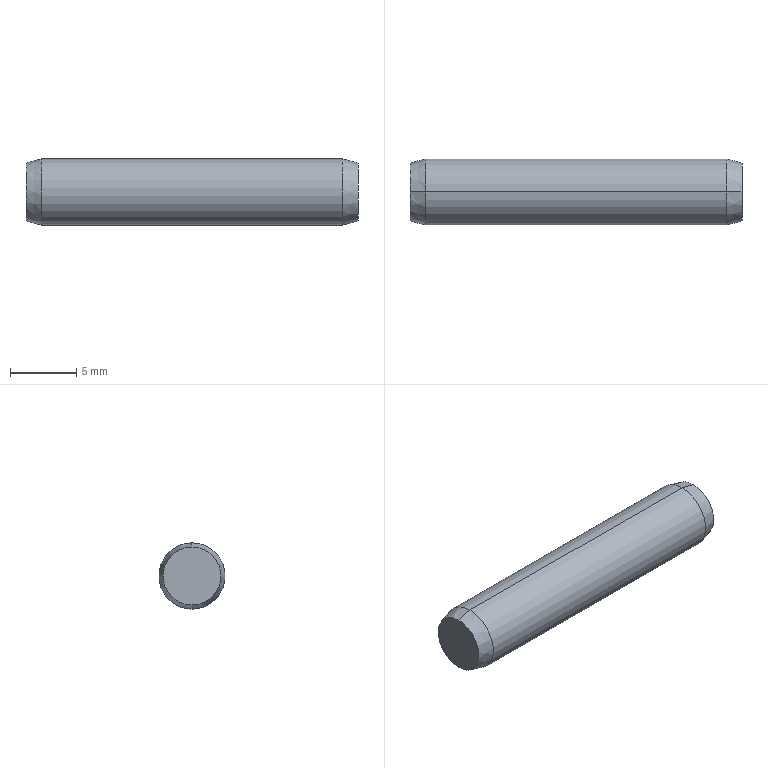Part | STEP file | GB/T 119 5×25 | 1 solid | 8 faces | box 25 x 5 x 5 mm | volume 485.073 mm3 | cone 4 | cylinder 2 | plane 2 | commonest cylinder face diameters 5 x2
STEP:
#1=CARTESIAN_POINT('',(21.6,0.,2.5));
#2=VERTEX_POINT('',#1);
#3=CARTESIAN_POINT('',(21.6,0.,-2.5));
#4=VERTEX_POINT('',#3);
#5=CARTESIAN_POINT('',(21.6,0.,0.));
#6=DIRECTION('',(-1.,0.,0.));
#7=DIRECTION('',(0.,0.,1.));
#8=AXIS2_PLACEMENT_3D('',#5,#6,#7);
#9=CIRCLE('',#8,2.5);
#10=EDGE_CURVE('',#2,#4,#9,.T.);
#11=ORIENTED_EDGE('',*,*,#10,.T.);
#12=CARTESIAN_POINT('',(-1.,0.,-2.5));
#13=VERTEX_POINT('',#12);
#14=CARTESIAN_POINT('',(0.,0.,-2.5));
#15=DIRECTION('',(-1.,0.,0.));
#16=VECTOR('',#15,1000.);
#17=LINE('',#14,#16);
#18=EDGE_CURVE('',#4,#13,#17,.T.);
#19=ORIENTED_EDGE('',*,*,#18,.T.);
#20=CARTESIAN_POINT('',(-1.,0.,2.5));
#21=VERTEX_POINT('',#20);
#22=CARTESIAN_POINT('',(-1.,0.,0.));
#23=DIRECTION('',(-1.,0.,0.));
#24=DIRECTION('',(0.,0.,1.));
#25=AXIS2_PLACEMENT_3D('',#22,#23,#24);
#26=CIRCLE('',#25,2.5);
#27=EDGE_CURVE('',#21,#13,#26,.T.);
#28=ORIENTED_EDGE('',*,*,#27,.F.);
#29=CARTESIAN_POINT('',(0.,0.,2.5));
#30=DIRECTION('',(-1.,0.,0.));
#31=VECTOR('',#30,1000.);
#32=LINE('',#29,#31);
#33=EDGE_CURVE('',#2,#21,#32,.T.);
#34=ORIENTED_EDGE('',*,*,#33,.F.);
#35=EDGE_LOOP('',(#11,#19,#28,#34));
#36=FACE_OUTER_BOUND('',#35,.T.);
#37=CARTESIAN_POINT('',(0.,0.,0.));
#38=DIRECTION('',(-1.,0.,0.));
#39=DIRECTION('',(0.,0.,1.));
#40=AXIS2_PLACEMENT_3D('',#37,#38,#39);
#41=CYLINDRICAL_SURFACE('',#40,2.5);
#42=ADVANCED_FACE('',(#36),#41,.T.);
#43=CARTESIAN_POINT('',(-2.2,0.,2.178));
#44=VERTEX_POINT('',#43);
#45=CARTESIAN_POINT('',(-2.2,0.,-2.178));
#46=VERTEX_POINT('',#45);
#47=CARTESIAN_POINT('',(-2.2,0.,0.));
#48=DIRECTION('',(-1.,0.,0.));
#49=DIRECTION('',(0.,0.,1.));
#50=AXIS2_PLACEMENT_3D('',#47,#48,#49);
#51=CIRCLE('',#50,2.178);
#52=EDGE_CURVE('',#44,#46,#51,.T.);
#53=ORIENTED_EDGE('',*,*,#52,.F.);
#54=CARTESIAN_POINT('',(-1.,0.,2.5));
#55=DIRECTION('',(0.9659,0.,0.2588));
#56=VECTOR('',#55,1000.);
#57=LINE('',#54,#56);
#58=EDGE_CURVE('',#44,#21,#57,.T.);
#59=ORIENTED_EDGE('',*,*,#58,.T.);
#60=ORIENTED_EDGE('',*,*,#27,.T.);
#61=CARTESIAN_POINT('',(-1.,0.,-2.5));
#62=DIRECTION('',(0.9659,0.,-0.2588));
#63=VECTOR('',#62,1000.);
#64=LINE('',#61,#63);
#65=EDGE_CURVE('',#46,#13,#64,.T.);
#66=ORIENTED_EDGE('',*,*,#65,.F.);
#67=EDGE_LOOP('',(#53,#59,#60,#66));
#68=FACE_OUTER_BOUND('',#67,.T.);
#69=CARTESIAN_POINT('',(-1.,0.,0.));
#70=DIRECTION('',(1.,0.,0.));
#71=DIRECTION('',(0.,0.,-1.));
#72=AXIS2_PLACEMENT_3D('',#69,#70,#71);
#73=CONICAL_SURFACE('',#72,2.5,0.2618);
#74=ADVANCED_FACE('',(#68),#73,.T.);
#75=CARTESIAN_POINT('',(22.8,0.,2.178));
#76=VERTEX_POINT('',#75);
#77=CARTESIAN_POINT('',(22.8,0.,-2.178));
#78=VERTEX_POINT('',#77);
#79=CARTESIAN_POINT('',(22.8,0.,0.));
#80=DIRECTION('',(-1.,0.,0.));
#81=DIRECTION('',(0.,0.,1.));
#82=AXIS2_PLACEMENT_3D('',#79,#80,#81);
#83=CIRCLE('',#82,2.178);
#84=EDGE_CURVE('',#76,#78,#83,.T.);
#85=ORIENTED_EDGE('',*,*,#84,.T.);
#86=CARTESIAN_POINT('',(22.8,0.,-2.178));
#87=DIRECTION('',(-0.9659,0.,-0.2588));
#88=VECTOR('',#87,1000.);
#89=LINE('',#86,#88);
#90=EDGE_CURVE('',#78,#4,#89,.T.);
#91=ORIENTED_EDGE('',*,*,#90,.T.);
#92=ORIENTED_EDGE('',*,*,#10,.F.);
#93=CARTESIAN_POINT('',(22.8,0.,2.178));
#94=DIRECTION('',(-0.9659,0.,0.2588));
#95=VECTOR('',#94,1000.);
#96=LINE('',#93,#95);
#97=EDGE_CURVE('',#76,#2,#96,.T.);
#98=ORIENTED_EDGE('',*,*,#97,.F.);
#99=EDGE_LOOP('',(#85,#91,#92,#98));
#100=FACE_OUTER_BOUND('',#99,.T.);
#101=CARTESIAN_POINT('',(22.8,0.,0.));
#102=DIRECTION('',(-1.,0.,0.));
#103=DIRECTION('',(0.,0.,1.));
#104=AXIS2_PLACEMENT_3D('',#101,#102,#103);
#105=CONICAL_SURFACE('',#104,2.178,0.2618);
#106=ADVANCED_FACE('',(#100),#105,.T.);
#107=ORIENTED_EDGE('',*,*,#90,.F.);
#108=CARTESIAN_POINT('',(22.8,0.,0.));
#109=DIRECTION('',(-1.,0.,0.));
#110=DIRECTION('',(0.,0.,1.));
#111=AXIS2_PLACEMENT_3D('',#108,#109,#110);
#112=CIRCLE('',#111,2.178);
#113=EDGE_CURVE('',#78,#76,#112,.T.);
#114=ORIENTED_EDGE('',*,*,#113,.T.);
#115=ORIENTED_EDGE('',*,*,#97,.T.);
#116=CARTESIAN_POINT('',(21.6,0.,0.));
#117=DIRECTION('',(-1.,0.,0.));
#118=DIRECTION('',(0.,0.,1.));
#119=AXIS2_PLACEMENT_3D('',#116,#117,#118);
#120=CIRCLE('',#119,2.5);
#121=EDGE_CURVE('',#4,#2,#120,.T.);
#122=ORIENTED_EDGE('',*,*,#121,.F.);
#123=EDGE_LOOP('',(#107,#114,#115,#122));
#124=FACE_OUTER_BOUND('',#123,.T.);
#125=CARTESIAN_POINT('',(22.8,0.,0.));
#126=DIRECTION('',(-1.,0.,0.));
#127=DIRECTION('',(0.,0.,1.));
#128=AXIS2_PLACEMENT_3D('',#125,#126,#127);
#129=CONICAL_SURFACE('',#128,2.178,0.2618);
#130=ADVANCED_FACE('',(#124),#129,.T.);
#131=ORIENTED_EDGE('',*,*,#84,.F.);
#132=ORIENTED_EDGE('',*,*,#113,.F.);
#133=EDGE_LOOP('',(#131,#132));
#134=FACE_OUTER_BOUND('',#133,.T.);
#135=CARTESIAN_POINT('',(22.8,2.178,0.));
#136=DIRECTION('',(-1.,0.,0.));
#137=DIRECTION('',(0.,0.,1.));
#138=AXIS2_PLACEMENT_3D('',#135,#136,#137);
#139=PLANE('',#138);
#140=ADVANCED_FACE('',(#134),#139,.F.);
#141=CARTESIAN_POINT('',(-2.2,0.,0.));
#142=DIRECTION('',(-1.,0.,0.));
#143=DIRECTION('',(0.,0.,1.));
#144=AXIS2_PLACEMENT_3D('',#141,#142,#143);
#145=CIRCLE('',#144,2.178);
#146=EDGE_CURVE('',#46,#44,#145,.T.);
#147=ORIENTED_EDGE('',*,*,#146,.T.);
#148=ORIENTED_EDGE('',*,*,#52,.T.);
#149=EDGE_LOOP('',(#147,#148));
#150=FACE_OUTER_BOUND('',#149,.T.);
#151=CARTESIAN_POINT('',(-2.2,2.178,0.));
#152=DIRECTION('',(1.,0.,0.));
#153=DIRECTION('',(0.,0.,-1.));
#154=AXIS2_PLACEMENT_3D('',#151,#152,#153);
#155=PLANE('',#154);
#156=ADVANCED_FACE('',(#150),#155,.F.);
#157=ORIENTED_EDGE('',*,*,#58,.F.);
#158=ORIENTED_EDGE('',*,*,#146,.F.);
#159=ORIENTED_EDGE('',*,*,#65,.T.);
#160=CARTESIAN_POINT('',(-1.,0.,0.));
#161=DIRECTION('',(-1.,0.,0.));
#162=DIRECTION('',(0.,0.,1.));
#163=AXIS2_PLACEMENT_3D('',#160,#161,#162);
#164=CIRCLE('',#163,2.5);
#165=EDGE_CURVE('',#13,#21,#164,.T.);
#166=ORIENTED_EDGE('',*,*,#165,.T.);
#167=EDGE_LOOP('',(#157,#158,#159,#166));
#168=FACE_OUTER_BOUND('',#167,.T.);
#169=CARTESIAN_POINT('',(-1.,0.,0.));
#170=DIRECTION('',(1.,0.,0.));
#171=DIRECTION('',(0.,0.,-1.));
#172=AXIS2_PLACEMENT_3D('',#169,#170,#171);
#173=CONICAL_SURFACE('',#172,2.5,0.2618);
#174=ADVANCED_FACE('',(#168),#173,.T.);
#175=ORIENTED_EDGE('',*,*,#18,.F.);
#176=ORIENTED_EDGE('',*,*,#121,.T.);
#177=ORIENTED_EDGE('',*,*,#33,.T.);
#178=ORIENTED_EDGE('',*,*,#165,.F.);
#179=EDGE_LOOP('',(#175,#176,#177,#178));
#180=FACE_OUTER_BOUND('',#179,.T.);
#181=CARTESIAN_POINT('',(0.,0.,0.));
#182=DIRECTION('',(-1.,0.,0.));
#183=DIRECTION('',(0.,0.,1.));
#184=AXIS2_PLACEMENT_3D('',#181,#182,#183);
#185=CYLINDRICAL_SURFACE('',#184,2.5);
#186=ADVANCED_FACE('',(#180),#185,.T.);
#187=CLOSED_SHELL('',(#42,#74,#106,#130,#140,#156,#174,#186));
#188=MANIFOLD_SOLID_BREP('',#187);
#189=CARTESIAN_POINT('',(0.,0.,0.));
#190=DIRECTION('',(0.,0.,1.));
#191=DIRECTION('',(1.,0.,0.));
#192=AXIS2_PLACEMENT_3D('',#189,#190,#191);
#193=(LENGTH_UNIT()NAMED_UNIT(*)SI_UNIT(.MILLI.,.METRE.));
#194=UNCERTAINTY_MEASURE_WITH_UNIT(LENGTH_MEASURE(0.00001),#193,'','');
#195=(NAMED_UNIT(*)PLANE_ANGLE_UNIT()SI_UNIT($,.RADIAN.));
#196=(NAMED_UNIT(*)SI_UNIT($,.STERADIAN.)SOLID_ANGLE_UNIT());
#197=(GEOMETRIC_REPRESENTATION_CONTEXT(3)GLOBAL_UNCERTAINTY_ASSIGNED_CONTEXT((#194))GLOBAL_UNIT_ASSIGNED_CONTEXT((#193,#195,#196))REPRESENTATION_CONTEXT('',''));
#198=ADVANCED_BREP_SHAPE_REPRESENTATION('',(#188,#192),#197);